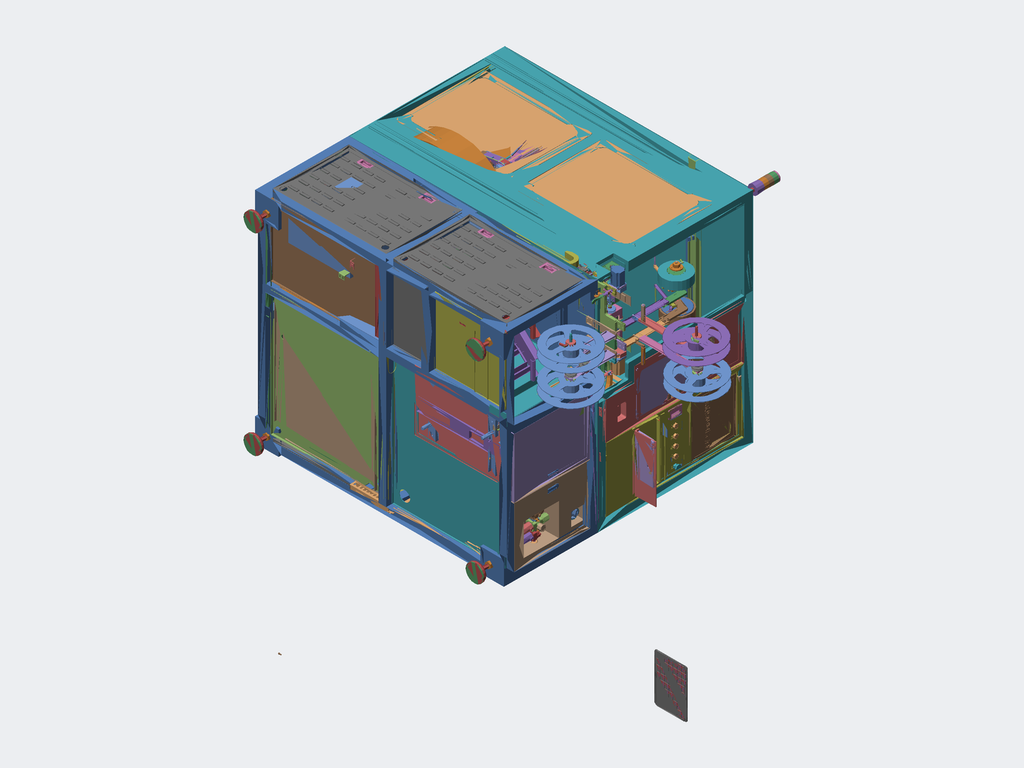Assembly | STEP file | 717 different items | 1668 placed
Parts list (item | name | quantity | parent item | size | volume), first 404 of 717 items:
1 | 11- Drag Chain 202811_2 | x3 | in 11-°ü×°11 | - | -
2 | 11- Filter C11 | x1 | - | - | -
3 | 11- M3-25 Hex Socket Countersunk Screw11_BOX-CBF3-25 | x1 | - | - | -
4 | 11- M3-5 Hex Socket Round Head Screw11_BCB3-5 | x5 | - | - | -
5 | 11- M4-10 Hex Socket Countersunk Screw11_BOX-CBF4-10 | x1 | - | - | -
6 | 11- M4-12 Hex Socket Countersunk Screw11_BOX-CBF4-12 | x2 | - | - | -
7 | 11- M4-20 Hex Socket Countersunk Screw11_BOX-CBF4-20 | x1 | - | - | -
8 | 11- M5 Nut CW11 | x2 | - | - | -
9 | 11- M5-12 Hex Socket Countersunk Screw11_BOX-CBF5-12 | x1 | - | - | -
10 | 11- M5-15 Hex Socket Countersunk Screw11_BOX-CBF5-15 | x1 | - | - | -
11 | 11- M5-30 Hex Socket Countersunk Screw11_BOX-CBF5-30 | x1 | - | - | -
12 | 11- M5-40 Hex Socket Countersunk Screw CW11_BOX-CBF5-40 | x2 | - | - | -
13 | 11- M5-40 Hex Socket Countersunk Screw11_BOX-CBF5-40 | x2 | - | - | -
14 | 11- M6-40 Hex Socket Countersunk Screw11_BOX-CBF6-40 | x1 | - | - | -
15 | 11- Mirror 99-JX-009-98-9865-998-1.·11 | x1 | - | - | -
16 | 11- Mirror 99-UWUAN94_B-98-9865-998-1.·11_UWUAN94-B | x1 | - | - | -
17 | 11- Mirror 99-XJX-006-98-9865-998-1.·11 | x1 | - | - | -
18 | 11- Mirror AJST4-5511 | x2 | - | - | -
19 | 11- Mirror ARM_MC01-S311 | x1 | in 11- Mirror MC01-S311 | - | -
20 | 11- Mirror AWY6_2511 | x1 | - | - | -
21 | 11- Mirror B676ZZ11_B676ZZ | x1 | - | - | -
22 | 11- Mirror B6800ZZ11_B6800ZZ | x4 | - | - | -
23 | 11- Mirror B686ZZ11_B686ZZ | x1 | - | - | -
24 | 11- Mirror B688ZZ11 | x2 | in 11- Mirror Roller111 | - | -
25 | 11- Mirror B698ZZ11_B698ZZ | x1 | - | - | -
26 | 11- Mirror BASE_MC01-S311 | x1 | in 11- Mirror MC01-S311 | - | -
27 | 11- Mirror BSPO4_15b11 | x2 | in 11- Mirror BSPO4_1511, 11- Mirror BSPO4_15111 | - | -
28 | 11- Mirror BZ-00811 | x1 | - | - | -
29 | 11- Mirror Body_A_CDQSB16_10D_A93_0_11 | x2 | in 11- Mirror CDQ16-10D11, 11- Mirror CDQ16-10D111 | - | -
30 | 11- Mirror CC-MCH-6.5-50-100-100w-6-5011 | x2 | - | - | -
31 | 11- Mirror CLDMC6_20_B_111 | x2 | in 11- Mirror CLDMC6_20_B11, 11- Mirror CLDMC6_20_B111 | - | -
32 | 11- Mirror CLDMC6_20_B_211 | x2 | in 11- Mirror CLDMC6_20_B11, 11- Mirror CLDMC6_20_B111 | - | -
33 | 11- Mirror CLMPLV_CLDM5-25-B11 | x2 | in 11- Mirror CLDM5-25-B11, 11- Mirror CLDM5-25-B111 | - | -
34 | 11- Mirror CLMP_MC01-S311 | x2 | in 11- Mirror MC01-S311 | - | -
35 | 11- Mirror FG-B00111 | x1 | - | - | -
36 | 11- Mirror FG-B00211 | x2 | - | - | -
37 | 11- Mirror FG-B00311 | x3 | - | - | -
38 | 11- Mirror FG-B00411 | x3 | - | - | -
39 | 11- Mirror FG-B00511 | x1 | - | - | -
40 | 11- Mirror FG-B00611 | x2 | - | - | -
41 | 11- Mirror FG-B00811 | x1 | - | - | -
42 | 11- Mirror FG-B00911 | x1 | - | - | -
43 | 11- Mirror FG-B01011 | x1 | - | - | -
44 | 11- Mirror FG-B01111 | x2 | - | - | -
45 | 11- Mirror FG-B01211 | x1 | - | - | -
46 | 11- Mirror FG-B01311 | x2 | - | - | -
47 | 11- Mirror FG-B01411 | x1 | - | - | -
48 | 11- Mirror FG-B01611 | x2 | - | - | -
49 | 11- Mirror FG-B01711 | x2 | - | - | -
50 | 11- Mirror FG-B01811 | x1 | - | - | -
51 | 11- Mirror FG-B01911 | x3 | - | - | -
52 | 11- Mirror FG-B02011 | x2 | - | - | -
53 | 11- Mirror FG-B02111 | x2 | - | - | -
54 | 11- Mirror FG-B02211 | x2 | - | - | -
55 | 11- Mirror FG-B02311 | x2 | - | - | -
56 | 11- Mirror FG-B02411 | x2 | - | - | -
57 | 11- Mirror FG-B02511 | x2 | - | - | -
58 | 11- Mirror FG-B02611 | x2 | - | - | -
59 | 11- Mirror FG-B02711 | x2 | - | - | -
60 | 11- Mirror FG-B02811 | x2 | - | - | -
61 | 11- Mirror FG-B03011 | x2 | - | - | -
62 | 11- Mirror FG-B03211 | x2 | - | - | -
63 | 11- Mirror FG-B03311 | x1 | - | - | -
64 | 11- Mirror FG-B03411 | x2 | - | - | -
65 | 11- Mirror FG-B03611 | x1 | - | - | -
66 | 11- Mirror FG-B03711 | x1 | - | - | -
67 | 11- Mirror FG-B03811 | x1 | - | - | -
68 | 11- Mirror FG-B03911 | x1 | - | - | -
69 | 11- Mirror FG-B04011 | x1 | - | - | -
70 | 11- Mirror FG-B04111 | x1 | - | - | -
71 | 11- Mirror FG-B04211 | x1 | - | - | -
72 | 11- Mirror FG-B04311 | x1 | - | - | -
73 | 11- Mirror FG-B04411 | x1 | - | - | -
74 | 11- Mirror FG-B04511 | x1 | - | - | -
75 | 11- Mirror FG-B04611 | x1 | - | - | -
76 | 11- Mirror FG-B04711 | x1 | - | - | -
77 | 11- Mirror FG-B04811 | x1 | - | - | -
78 | 11- Mirror FG-B04911 | x1 | - | - | -
79 | 11- Mirror FG-B05011 | x1 | - | - | -
80 | 11- Mirror FG-B05111 | x1 | - | - | -
81 | 11- Mirror FG-B05211 | x1 | - | - | -
82 | 11- Mirror FG-B05311 | x1 | - | - | -
83 | 11- Mirror FG-B05411 | x1 | - | - | -
84 | 11- Mirror FG-B05511 | x1 | - | - | -
85 | 11- Mirror FG-B05611 | x1 | - | - | -
86 | 11- Mirror FG-B05711 | x1 | - | - | -
87 | 11- Mirror FG-B05811 | x1 | - | - | -
88 | 11- Mirror FG-B05911 | x2 | - | - | -
89 | 11- Mirror FG-B06011 | x1 | - | - | -
90 | 11- Mirror FG-B06711 | x1 | - | - | -
91 | 11- Mirror FG-B06811 | x1 | in 11- Mirror Roller111 | - | -
92 | 11- Mirror FG-B06911 | x1 | in 11- Mirror Roller111 | - | -
93 | 11- Mirror FG-B07111 | x3 | - | - | -
94 | 11- Mirror FG-B07211 | x1 | - | - | -
95 | 11- Mirror FG-B07311 | x1 | - | - | -
96 | 11- Mirror FG-B07411 | x1 | - | - | -
97 | 11- Mirror FG-B07511 | x2 | - | - | -
98 | 11- Mirror FG-B07611 | x2 | - | - | -
99 | 11- Mirror FG-B07711 | x1 | - | - | -
100 | 11- Mirror FG-B07811 | x2 | - | - | -
101 | 11- Mirror FG-B07911 | x1 | - | - | -
102 | 11- Mirror FG-B08011 | x2 | - | - | -
103 | 11- Mirror FG-B08111 | x1 | - | - | -
104 | 11- Mirror FG-B08211 | x2 | - | - | -
105 | 11- Mirror FG-B08311 | x1 | - | - | -
106 | 11- Mirror FG-B08611 | x1 | - | - | -
107 | 11- Mirror FG-B08711 | x2 | - | - | -
108 | 11- Mirror FG-B08811 | x1 | - | - | -
109 | 11- Mirror FG-B08911 | x1 | - | - | -
110 | 11- Mirror FG-BZ02111 | x1 | - | - | -
111 | 11- Mirror FG-BZ02211 | x1 | - | - | -
112 | 11- Mirror FG-BZ02311 | x1 | - | - | -
113 | 11- Mirror FG-BZ02411 | x1 | - | - | -
114 | 11- Mirror FG-BZ02511 | x1 | - | - | -
115 | 11- Mirror FG-SB00411 | x1 | in 11- Media Pick-up Nozzle Assembly-A11 | - | -
116 | 11- Mirror FG-SB00511 | x1 | in 11- Media Pick-up Nozzle Assembly-A11 | - | -
117 | 11- Mirror FG-SB00611 | x1 | in 11- Media Pick-up Nozzle Assembly-A11 | - | -
118 | 11- Mirror FG-SB00711 | x3 | in 11- Media Pick-up Nozzle Assembly-A11 | - | -
119 | 11- Mirror FG-SB00811 | x1 | in 11- Media Pick-up Nozzle Assembly-A11 | - | -
120 | 11- Mirror FG-SB00911 | x1 | in 11- Media Pick-up Nozzle Assembly-A11 | - | -
121 | 11- Mirror FG-SZ01811 | x1 | - | - | -
122 | 11- Mirror FJTM4_0_7_413part111 | x2 | in 11- Mirror FJTM4_0_7_411, 11- Mirror FJTM4_0_7_4111 | - | -
123 | 11- Mirror FJTM4_0_7_413part211 | x2 | in 11- Mirror FJTM4_0_7_411, 11- Mirror FJTM4_0_7_4111 | - | -
124 | 11- Mirror FL6800ZZ11_FL6800ZZ | x2 | - | - | -
125 | 11- Mirror FL6902ZZ11 | x2 | - | - | -
126 | 11- Mirror GYJJ-013-q11 | x3 | - | - | -
127 | - | x4 | in 11- Mirror HTPA24S3M060_A_P811, 11- Mirror HTPA24S3M060_A_P8111 | - | -
128 | 11- Mirror HANDLE_MC01-S311 | x1 | in 11- Mirror MC01-S311 | - | -
129 | 11- Mirror HGR1511 | x2 | in 11- Mirror HGW15CC11, 11- Mirror HGW15CC111 | - | -
130 | 11- Mirror HGW1511 | x4 | in 11- Mirror HGW15CC11, 11- Mirror HGW15CC111 | - | -
131 | 11- Mirror HLB1011_HLB10 | x1 | - | - | -
132 | 11- Mirror HTPA24S3M060_A_P8_a11 | x2 | in 11- Mirror HTPA24S3M060_A_P811, 11- Mirror HTPA24S3M060_A_P8111 | - | -
133 | 11- Mirror KEYENCE-PQ0211 | x2 | - | - | -
134 | 11- Mirror LINK_MC01-S311 | x1 | in 11- Mirror MC01-S311 | - | -
135 | 11- Mirror LMU6-A11_C-LMU6 | x3 | in 11- Media Pick-up Nozzle Assembly-A11 | - | -
136 | 11- Mirror LMU_N811 | x3 | - | - | -
137 | 11- Mirror M3-25 Hex Socket Countersunk Screw11_BOX-CBF3-25 | x1 | - | - | -
138 | 11- Mirror M3-5 Hex Socket Round Head Screw11_BCB3-5 | x5 | - | - | -
139 | 11- Mirror M4x0_7A11 | x2 | in 11- Mirror BSPO4_1511, 11- Mirror BSPO4_15111 | - | -
140 | 11- Mirror M5-15 Hex Socket Countersunk Screw11_BOX-CBF5-15 | x1 | - | - | -
141 | 11- Mirror M5-40 Hex Socket Countersunk Screw11_BOX-CBF5-40 | x2 | - | - | -
142 | 11- Mirror M6-40 Hex Socket Countersunk Screw11_BOX-CBF6-40 | x1 | - | - | -
143 | 11- Mirror MANIFOLD_SOLID_BREP_3911 | x6 | in 11- Mirror SAND94F7H98T_ASM11, 11- Mirror SAND94F7H98T_ASM111 | - | -
144 | 11- Mirror MANIFOLD_SOLID_BREP_4011 | x2 | in 11- Mirror SAND94F7H98T_ASM11, 11- Mirror SAND94F7H98T_ASM111 | - | -
145 | 11- Mirror MBR58_3_P811 | x2 | - | - | -
146 | 11- Mirror MSB6_2011 | x1 | - | - | -
147 | 11- Mirror MSB8_1011_MSB8-10 | x1 | - | - | -
148 | 11- Mirror Mirror FG-B01911 | x1 | - | - | -
149 | 11- Mirror Mirror FG-B07111 | x1 | - | - | -
150 | 11- Mirror Mirror FG-B07511 | x1 | - | - | -
151 | 11- Mirror Mirror FG-B07611 | x1 | - | - | -
152 | 11- Mirror NAT-M6_MC01-S311 | x2 | in 11- Mirror MC01-S311 | - | -
153 | 11- Mirror NEZI-M6x40L_MC01-S311 | x1 | in 11- Mirror MC01-S311 | - | -
154 | 11- Mirror NEZIPART_CLDM5-25-B11 | x2 | in 11- Mirror CLDM5-25-B11, 11- Mirror CLDM5-25-B111 | - | -
155 | 11- Mirror Rod_A_CDQSB16_10D_A93_0_11 | x2 | in 11- Mirror CDQ16-10D11, 11- Mirror CDQ16-10D111 | - | -
156 | 11- Mirror SFJW6-31-M3-N311 | x3 | in 11- Media Pick-up Nozzle Assembly-A11 | - | -
157 | 11- Mirror SSEBT13_7011 | x2 | in 11- Mirror SSEBT13-7011 | - | -
158 | 11- Mirror STWN1511 | x1 | - | - | -
159 | 11- Mirror STWN811 | x2 | in 11- Mirror Roller111 | - | -
160 | 11- Mirror UF8-15-A11_UV8-15 | x1 | in 11- Media Pick-up Nozzle Assembly-A11 | - | -
161 | 11- Mirror WT8_1511 | x1 | - | - | -
162 | 11- Mirror b_SEB1011 | x2 | in 11- Mirror SEBL10_4011, 11- Mirror SEBL10_40111 | - | -
163 | 11- Mirror b_SSEBT1311 | x2 | in 11- Mirror SSEBT13-7011 | - | -
164 | 11- Mirror c-ssmt6-100011 | x2 | - | - | -
165 | 11- Mirror r_SEBL10_4011 | x2 | in 11- Mirror SEBL10_4011, 11- Mirror SEBL10_40111 | - | -
166 | 11- Mirror roller-HSG11 | x2 | - | - | -
167 | 11- Mirror yk60hb86-04a11 | x1 | - | - | -
168 | 11- Optics Valley MISUMI-KES3-1511 | x1 | - | - | -
169 | 11- Optics Valley SS11111 | x2 | - | - | -
170 | 11- Optics Valley SS11411 | x1 | - | - | -
171 | 11-100GF-RC11 | x1 | in 11-200YB03_ASM-111 | 159.399 x 104.797 x 116.9 mm | 1389549 mm3
172 | 11-100YB200G11 | x1 | in 11-200YB03_ASM-111 | 105.972 x 105.485 x 221 mm | 385712 mm3
173 | 11-123211 | x2 | - | 450 x 380 x 10 mm | 1708660 mm3
174 | - | x1 | - | 80 x 80 x 151 mm | 637905 mm3
175 | - | x1 | - | - | -
176 | 11-6060-21411 | x1 | - | 62 x 44 x 264 mm | 101240 mm3
177 | - | x1 | - | - | -
178 | - | x1 | - | - | -
179 | - | x1 | - | - | -
180 | - | x1 | - | - | -
181 | - | x1 | - | - | -
182 | - | x2 | in 11-COMPANY_A Upper Frame Cover.·11 | 50 x 10 x 14 mm | 4964 mm3
183 | - | x2 | in 11-COMPANY_A Upper Frame Cover.·11 | 50 x 14 x 14 mm | 5525 mm3
184 | - | x1 | - | - | -
185 | - | x1 | in 11-COMPANY_A Upper Frame Cover.·11 | - | -
186 | 11-ACA-0806-1_BodyCW11_HI | x2 | in 11-ACA-0806-1CW11_HI | 8 x 50 x 8 mm | 1845 mm3
187 | 11-ACA-0806-1_NTCW11_HI | x4 | in 11-ACA-0806-1CW11_HI | 11 x 4 x 12.325 mm | 245.478 mm3
188 | 11-ACA2020-311 | x4 | - | 26 x 127.5 x 29.132 mm | 35458 mm3
189 | 11-AJST4-5511 | x2 | - | 70 x 8.083 x 7 mm | 1036 mm3
190 | 11-ARM_MC01-S311 | x1 | in 11-MC01-S311 | 68.35 x 24.739 x 11.4 mm | 4057 mm3
191 | 11-ASL5-M511 | x1 | - | 28.6 x 30 x 12.5 mm | 2571 mm3
192 | 11-AWY6_2511 | x1 | - | 26.2 x 6 x 6 mm | 169.712 mm3
193 | 11-B6800ZZ11_B6800ZZ | x2 | - | 5 x 19 x 19 mm | 1010 mm3
194 | 11-B686ZZ11_B686ZZ | x2 | in 11-°ü×°11 | 5 x 13 x 13 mm | 508.574 mm3
195 | 11-B688ZZ11 | x2 | in 11-Roller11 | 5 x 16 x 16 mm | 730.663 mm3
196 | 11-B6902ZZ11_B6902ZZ | x2 | - | 7 x 28 x 28 mm | 2801 mm3
197 | 11-B698ZZ11_B698ZZ | x1 | - | 6 x 19 x 19 mm | 1232 mm3
198 | 11-BASE_MC01-S311 | x1 | in 11-MC01-S311 | 37 x 25.5 x 36 mm | 4977 mm3
199 | 11-BSPO4_15b11 | x2 | in 11-BSPO4_1511 | 15 x 4 x 4 mm | 171.383 mm3
200 | 11-Base1111 | x2 | - | 290.067 x 170 x 310 mm | 1578242 mm3
201 | 11-Body_A_CDQSB16_10D_A93_0_11 | x2 | in 11-CDQ16-10D11 | 29 x 29 x 32 mm | 21093 mm3
202 | 11-CB5_15_1-ab11 | x18 | in 11-KDST12-ab11_KDST12 | 20 x 8.5 x 8.5 mm | 539.598 mm3
203 | 11-CC-MCH-6.5-50-100-100w-6-5011 | x2 | - | 6.5 x 6.5 x 70 mm | 1785 mm3
204 | 11-CLDMC6_20_B_111 | x4 | in 11-CLDMC6_20_B11 | 10 x 45.8 x 10 mm | 2201 mm3
205 | 11-CLDMC6_20_B_211 | x4 | in 11-CLDMC6_20_B11 | 36.5 x 25 x 13 mm | 3149 mm3
206 | 11-CLMPLV_CLDM5-25-B11 | x2 | in 11-CLDM5-25-B11 | 51.5 x 31 x 13 mm | 5282 mm3
207 | 11-CLMP_MC01-S311 | x2 | in 11-MC01-S311 | 18.4 x 3.9 x 15.2 mm | 446.915 mm3
208 | 11-CX-442 (Panasonic)11 | x2 | - | - | -
209 | 11-Cover11111 | x2 | - | - | -
210 | 11-Cover21111 | x2 | - | 305.265 x 4 x 124.613 mm | 9765 mm3
211 | 11-Cover31111 | x2 | - | 105.323 x 67.359 x 38.98 mm | 17481 mm3
212 | 11-Cover41111 | x2 | - | 127.366 x 293 x 68 mm | 86944 mm3
213 | 11-DHJ-LR-144X1911 | x4 | - | 144 x 19 x 41 mm | 51924 mm3
214 | 11-EE-SX674A11 | x3 | - | 13.6 x 27.7 x 15.5 mm | 2495 mm3
215 | 11-EG15_RAIL_170CW11 | x1 | in 11-EGH15CA1R200ZOC11 | 15 x 12.5 x 200 mm | 31138 mm3
216 | 11-EGH15CA_BLOCK_2CW11 | x2 | in 11-EGH15CA1R200ZOC11 | 34 x 19.5 x 56.8 mm | 30383 mm3
217 | 11-F-ACA10LM11 | x2 | - | 15.4 x 16 x 14 mm | 1343 mm3
218 | 11-F12906-LQ-STBB5_35bA11 | x3 | - | 38.5 x 9.2 x 8 mm | 847.17 mm3
219 | 11-F12906-LQ-XZQG1A11 | x2 | in 11-F12906-LQ-AIRTAC-HRQ30-A-G(DS1-H)A11 | 195.5 x 57 x 191 mm | 392334 mm3
220 | 11-F12906-LQ-XZQG2A11 | x2 | in 11-F12906-LQ-AIRTAC-HRQ30-A-G(DS1-H)A11 | 42 x 4 x 5.1 mm | 360.74 mm3
221 | 11-F12906-LQ-XZQG3A11 | x2 | in 11-F12906-LQ-AIRTAC-HRQ30-A-G(DS1-H)A11 | 42 x 4 x 5.1 mm | 360.74 mm3
222 | 11-FCG-ZJ10011 | x1 | in 11-200YB03_ASM-111 | 19 x 64 x 64 mm | 16815 mm3
223 | 11-FG Emergency Stop Switch (Red) 22mm.11 | x1 | - | - | -
224 | 11-FG Guangyu2222AN-00311 | x1 | - | - | -
225 | 11-FG Push Button Switch (White) 22mm.11 | x4 | - | - | -
226 | 11-FG-00911 | x1 | in 11- Acrylic Door 2.·11 | 618 x 900 x 5 mm | 2751412 mm3
227 | 11-FG-01011 | x1 | - | 300 x 370 x 5 mm | 531993 mm3
228 | 11-FG-B00111 | x1 | - | 20 x 25 x 97.4 mm | 30314 mm3
229 | 11-FG-B00211 | x2 | - | 20 x 25 x 96.4 mm | 29627 mm3
230 | 11-FG-B00311 | x3 | - | 127 x 10 x 5 mm | 4266 mm3
231 | 11-FG-B00411 | x3 | - | 8 x 8 x 137 mm | 6844 mm3
232 | 11-FG-B00511 | x1 | - | 15 x 31 x 25 mm | 8369 mm3
233 | 11-FG-B00611 | x1 | - | 13.5 x 8.4 x 419 mm | 44557 mm3
234 | 11-FG-B00711 | x1 | - | 60 x 67.3 x 10 mm | 36302 mm3
235 | 11-FG-B00811 | x1 | - | 20 x 50 x 97.4 mm | 60152 mm3
236 | 11-FG-B00911 | x1 | - | 20 x 50 x 96.4 mm | 61320 mm3
237 | 11-FG-B01011 | x1 | - | 15 x 31 x 50 mm | 19389 mm3
238 | 11-FG-B01111 | x1 | - | 13.5 x 8.4 x 426 mm | 45040 mm3
239 | 11-FG-B01211 | x1 | - | 34 x 95 x 45 mm | 11150 mm3
240 | 11-FG-B01311 | x1 | - | 29 x 16.2 x 16.2 mm | 699.681 mm3
241 | 11-FG-B01411 | x1 | - | 8 x 21.5 x 55 mm | 827.809 mm3
242 | 11-FG-B01511 | x3 | - | 50 x 47.5 x 15 mm | 25829 mm3
243 | 11-FG-B01611 | x2 | - | 11 x 10 x 17 mm | 1460 mm3
244 | 11-FG-B01711 | x2 | - | 4 x 4 x 155 mm | 1945 mm3
245 | 11-FG-B01811 | x1 | - | 127 x 237 x 10 mm | 161294 mm3
246 | 11-FG-B01911 | x1 | - | 165 x 10 x 65 mm | 66276 mm3
247 | 11-FG-B02011 | x2 | - | 34 x 34 x 7 mm | 7241 mm3
248 | 11-FG-B02111 | x2 | - | 40.5 x 70 x 71 mm | 84307 mm3
249 | 11-FG-B02211 | x2 | - | 8 x 82 x 55 mm | 15645 mm3
250 | 11-FG-B02311 | x2 | - | 14 x 55 x 108 mm | 52508 mm3
251 | 11-FG-B02411 | x2 | - | 53 x 9 x 15 mm | 5874 mm3
252 | 11-FG-B02511 | x2 | - | 50 x 55 x 30 mm | 33514 mm3
253 | 11-FG-B02611 | x2 | - | 70 x 8 x 8 mm | 2907 mm3
254 | 11-FG-B02711 | x2 | - | 55 x 24 x 25 mm | 23943 mm3
255 | 11-FG-B02811 | x2 | - | 55 x 25 x 8 mm | 9529 mm3
256 | 11-FG-B02911 | x1 | - | 20 x 25 x 97.4 mm | 29767 mm3
257 | 11-FG-B03011 | x2 | - | 55 x 30 x 6 mm | 6845 mm3
258 | 11-FG-B03111 | x1 | - | 1.6 x 16 x 110 mm | 2770 mm3
259 | 11-FG-B03211 | x2 | - | 18.5 x 14.8 x 55 mm | 13198 mm3
260 | 11-FG-B03311 | x2 | - | 32 x 55 x 25 mm | 31224 mm3
261 | 11-FG-B03411 | x2 | - | 73 x 164 x 62 mm | 23088 mm3
262 | 11-FG-B03511 | x1 | - | 60 x 67.3 x 10 mm | 35980 mm3
263 | 11-FG-B03611 | x1 | - | 35 x 90 x 10 mm | 26239 mm3
264 | 11-FG-B03711 | x1 | - | 60 x 69.55 x 10 mm | 25100 mm3
265 | 11-FG-B03811 | x1 | - | 46 x 20 x 9 mm | 5580 mm3
266 | 11-FG-B03911 | x1 | - | 70 x 15 x 10.45 mm | 9294 mm3
267 | 11-FG-B04011 | x1 | - | 13 x 13 x 12.6 mm | 939.65 mm3
268 | 11-FG-B04111 | x1 | - | 30 x 30 x 15 mm | 6699 mm3
269 | 11-FG-B04211 | x1 | - | 13 x 13 x 19 mm | 1362 mm3
270 | 11-FG-B04311 | x1 | - | 13 x 13 x 2 mm | 108.385 mm3
271 | 11-FG-B04411 | x1 | - | 16 x 193.5 x 14 mm | 10709 mm3
272 | 11-FG-B045-(Standard Gear)11 | x2 | - | - | -
273 | 11-FG-B04611 | x2 | - | 35 x 35 x 16 mm | 6298 mm3
274 | 11-FG-B04711 | x1 | - | 100 x 40 x 12 mm | 42920 mm3
275 | 11-FG-B04811 | x1 | - | 40 x 300 x 10 mm | 115513 mm3
276 | 11-FG-B04911 | x1 | - | 107.65 x 192.793 x 12 mm | 106173 mm3
277 | 11-FG-B05011 | x1 | - | 9.8 x 44.825 x 230.182 mm | 35809 mm3
278 | 11-FG-B05111 | x1 | - | 6 x 6 x 135 mm | 3802 mm3
279 | 11-FG-B05211 | x1 | - | 50 x 45 x 12 mm | 12836 mm3
280 | 11-FG-B05311 | x1 | - | 160 x 160 x 5 mm | 93587 mm3
281 | 11-FG-B05411 | x1 | - | 76 x 76 x 19 mm | 36918 mm3
282 | 11-FG-B05511 | x1 | - | 90 x 90 x 10 mm | 52768 mm3
283 | 11-FG-B05611 | x1 | - | 66 x 66 x 25 mm | 31855 mm3
284 | 11-FG-B05711 | x1 | - | 20 x 20 x 147 mm | 20612 mm3
285 | 11-FG-B05811 | x1 | - | 40 x 400 x 12 mm | 182663 mm3
286 | 11-FG-B05911 | x3 | - | 50 x 47.5 x 9 mm | 15360 mm3
287 | 11-FG-B06011 | x3 | - | 20 x 20 x 169.5 mm | 19381 mm3
288 | 11-FG-B06111 | x2 | - | 40 x 200 x 10 mm | 76186 mm3
289 | 11-FG-B06211 | x2 | - | 60 x 300 x 12 mm | 199770 mm3
290 | 11-FG-B06611 | x2 | - | 40 x 20 x 10 mm | 5422 mm3
291 | 11-FG-B06711 | x1 | - | 80 x 12 x 10 mm | 7960 mm3
292 | 11-FG-B06811 | x1 | in 11-Roller11 | 20 x 20 x 100 mm | 19227 mm3
293 | 11-FG-B06911 | x1 | in 11-Roller11 | 8 x 8 x 111 mm | 5459 mm3
294 | 11-FG-B07111 | x1 | - | 29 x 11 x 19.5 mm | 3288 mm3
295 | 11-FG-B07211 | x1 | - | 240 x 1100 x 15 mm | 2663856 mm3
296 | 11-FG-B07311 | x2 | - | 15 x 80 x 73 mm | 13404 mm3
297 | 11-FG-B07411 | x1 | - | 265 x 317.5 x 137 mm | 178477 mm3
298 | 11-FG-B07511 | x1 | - | 14.5 x 6 x 419 mm | 26571 mm3
299 | 11-FG-B07611 | x1 | - | 14.5 x 6 x 369.8 mm | 23525 mm3
300 | 11-FG-B07711 | x1 | - | 8.2 x 40 x 20 mm | 919.559 mm3
301 | 11-FG-B07811 | x2 | - | 50.5 x 9.5 x 25 mm | 9037 mm3
302 | 11-FG-B07911 | x1 | - | 15 x 55 x 25 mm | 16309 mm3
303 | 11-FG-B08011 | x2 | - | 20 x 32.5 x 4 mm | 1470 mm3
304 | 11-FG-B08111 | x1 | - | 8.2 x 40 x 20 mm | 912.829 mm3
305 | 11-FG-B08211 | x2 | - | 10 x 35 x 3 mm | 935.086 mm3
306 | 11-FG-B08311 | x1 | - | 4 x 4 x 130 mm | 1631 mm3
307 | 11-FG-B08411 | x2 | - | 8 x 7 x 41 mm | 1772 mm3
308 | 11-FG-B08511 | x2 | - | 40 x 10 x 10 mm | 3274 mm3
309 | 11-FG-B08611 | x1 | - | 126 x 381.8 x 413.682 mm | 331589 mm3
310 | 11-FG-B08711 | x1 | in 11-°ü×°11 | 70 x 20 x 20 mm | 26205 mm3
311 | 11-FG-B08911 | x2 | in 11-°ü×°11 | 44 x 31 x 400 mm | 61704 mm3
312 | 11-FG-B09011 | x2 | in 11-°ü×°11 | 70 x 60 x 60 mm | 21228 mm3
313 | 11-FG-DB00111 | x1 | - | 1650 x 1450 x 20 mm | 31427316 mm3
314 | 11-FG-E00111 | x1 | - | 300 x 186 x 20 mm | 846486 mm3
315 | 11-FG-E00211 | x2 | - | 60 x 234 x 15 mm | 152627 mm3
316 | 11-FG-E00311 | x1 | - | 25 x 38 x 30 mm | 10262 mm3
317 | 11-FG-E00411 | x1 | - | 25 x 38 x 30 mm | 10226 mm3
318 | 11-FG-E00511 | x1 | - | 32 x 108 x 10 mm | 20715 mm3
319 | 11-FG-E00611 | x1 | - | 80 x 30 x 12 mm | 11899 mm3
320 | 11-FG-E00711 | x1 | - | 10 x 11.547 x 52 mm | 1820 mm3
321 | 11-FG-E00811 | x1 | - | 67 x 44 x 9 mm | 18765 mm3
322 | 11-FG-E00911 | x1 | - | 32 x 40 x 10 mm | 10413 mm3
323 | 11-FG-E01011 | x1 | - | 145 x 60 x 15 mm | 112264 mm3
324 | 11-FG-E01111 | x1 | - | 100 x 15 x 200 mm | 285807 mm3
325 | 11-FG-E01211 | x1 | - | 85 x 20 x 29 mm | 44302 mm3
326 | 11-FG-E01311 | x2 | - | 45 x 40 x 16 mm | 15803 mm3
327 | 11-FG-E01411 | x1 | - | 28 x 12 x 43 mm | 8595 mm3
328 | 11-FG-E01511 | x1 | - | 180 x 70 x 17 mm | 176306 mm3
329 | 11-FG-E01611 | x2 | - | 18 x 35 x 13 mm | 6444 mm3
330 | 11-FG-E01711 | x4 | - | 31.54 x 53.795 x 3 mm | 2242 mm3
331 | 11-FG-E01811 | x1 | - | 42 x 45 x 8 mm | 10535 mm3
332 | 11-FG-E01911 | x2 | - | 30 x 79.5 x 10 mm | 21106 mm3
333 | 11-FG-E02011 | x4 | - | 70 x 96 x 12 mm | 42748 mm3
334 | 11-FG-E02111 | x4 | - | 15 x 40 x 53 mm | 17580 mm3
335 | 11-FG-E02211 | x2 | - | 110 x 120 x 14.5 mm | 149751 mm3
336 | 11-FG-E02311 | x2 | - | 150 x 120 x 12 mm | 207598 mm3
337 | 11-FG-E02411 | x1 | - | 180 x 70 x 17 mm | 168926 mm3
338 | 11-FG-E02511 | x8 | - | 15 x 40 x 15 mm | 6347 mm3
339 | 11-FG-E02611 | x2 | - | 21 x 46 x 5 mm | 3756 mm3
340 | 11-FG-E02711 | x1 | - | 38.1 x 20.5 x 8.5 mm | 5078 mm3
341 | 11-FG-E02811 | x1 | - | 10 x 25 x 3.5 mm | 772.571 mm3
342 | 11-FG-E02911 | x1 | - | 304 x 110 x 150 mm | 146272 mm3
343 | 11-FG-E03011 | x1 | - | 113 x 304 x 128 mm | 112726 mm3
344 | 11-FG-E03111 | x1 | - | 140 x 100 x 2 mm | 20888 mm3
345 | 11-FG-E03211 | x1 | - | 88 x 17 x 26 mm | 5114 mm3
346 | 11-FG-E03311 | x2 | - | 41 x 169.5 x 10 mm | 55320 mm3
347 | 11-FG-E03411 | x1 | - | 48 x 47 x 8 mm | 12187 mm3
348 | 11-FG-E03511 | x1 | - | 33 x 20.5 x 8.5 mm | 4296 mm3
349 | 11-FG-E03611 | x1 | - | 55 x 54 x 27 mm | 21102 mm3
350 | 11-FG-E03711 | x1 | - | 20 x 20 x 119 mm | 14191 mm3
351 | 11-FG-E03811 | x1 | - | 86 x 120 x 10 mm | 47794 mm3
352 | 11-FG-E03911 | x4 | - | 12 x 12 x 53 mm | 5607 mm3
353 | 11-FG-E04111 | x1 | - | 24 x 28 x 5 mm | 1836 mm3
354 | 11-FG-E04211 | x1 | - | 32 x 51.5 x 15 mm | 7039 mm3
355 | 11-FG-E04311 | x1 | - | 40 x 10 x 10 mm | 3121 mm3
356 | 11-FG-E04411 | x1 | - | 28 x 12 x 35 mm | 10850 mm3
357 | 11-FG-E04511 | x1 | - | 8 x 40 x 20 mm | 5456 mm3
358 | 11-FG-E04611 | x4 | - | 15 x 14 x 3 mm | 458.934 mm3
359 | 11-FG-GD00111 | x4 | - | 64 x 71.5 x 15 mm | 48677 mm3
360 | 11-FG-JJ-01211 | x1 | - | 586 x 623 x 57 mm | 744145 mm3
361 | 11-FG-JX00111 | x1 | - | 408 x 519 x 20 mm | 549034 mm3
362 | 11-FG-JX00211 | x1 | - | 1500 x 667.5 x 1700 mm | 66450953 mm3
363 | 11-FG-JX00411 | x1 | - | 408 x 519 x 106 mm | 749356 mm3
364 | 11-FG-JX00511 | x1 | - | 100 x 20 x 138 mm | 43680 mm3
365 | 11-FG-JX00611 | x1 | in 11-COMPANY_A Upper Frame Cover.·11 | 1500 x 1700 x 1065 mm | 13737481 mm3
366 | 11-FG-JX01211 | x1 | in 11- Acrylic Door 2.·11 | 688 x 948 x 20 mm | 601333 mm3
367 | 11-FG-JX01311 | x1 | - | 240 x 460 x 10 mm | 240740 mm3
368 | 11-FG-JX01411 | x1 | - | 485 x 460 x 10 mm | 675418 mm3
369 | 11-FG-JX01511 | x1 | - | 775 x 890 x 10 mm | 929885 mm3
370 | 11-FG-JX01611 | x1 | - | 775 x 521 x 24.03 mm | 906085 mm3
371 | 11-FG-JX01711 | x1 | - | 358 x 948 x 37 mm | 620154 mm3
372 | 11-FG-JX01911 | x1 | - | 415 x 630 x 2 mm | 516605 mm3
373 | 11-FG-JX02011 | x1 | - | 302 x 556 x 460 mm | 760169 mm3
374 | 11-FG-S00111 | x5 | - | 12 x 12 x 260 mm | 29196 mm3
375 | 11-FG-S00211 | x5 | - | 12 x 12 x 180 mm | 20348 mm3
376 | 11-FG-S00311 | x4 | - | 148 x 23 x 32 mm | 9076 mm3
377 | 11-FG-S00411 | x4 | - | 12 x 12 x 190 mm | 19715 mm3
378 | 11-FG-S00511 | x4 | - | 40 x 52 x 10 mm | 16876 mm3
379 | 11-FG-S00611 | x6 | - | 48 x 35 x 46 mm | 33562 mm3
380 | 11-FG-S00711 | x3 | - | 69 x 35 x 38.6 mm | 65613 mm3
381 | 11-FG-S00811 | x3 | - | 98 x 100 x 76 mm | 565928 mm3
382 | 11-FG-S00911 | x1 | - | 420 x 15 x 110 mm | 675941 mm3
383 | 11-FG-S01011 | x1 | - | 140 x 70 x 15 mm | 110078 mm3
384 | 11-FG-S01111 | x1 | - | 80 x 17 x 110 mm | 120634 mm3
385 | 11-FG-S01211 | x1 | - | 120 x 15 x 57 mm | 50768 mm3
386 | 11-FG-S01311 | x2 | - | 60 x 15 x 120 mm | 30172 mm3
387 | 11-FG-S01411 | x1 | - | 69 x 35 x 75.5 mm | 96843 mm3
388 | 11-FG-S01511 | x1 | - | 160 x 15 x 90 mm | 120227 mm3
389 | 11-FG-S01611 | x3 | - | 180 x 20 x 30 mm | 87134 mm3
390 | 11-FG-S01711 | x2 | - | 20 x 580 x 20 mm | 181847 mm3
391 | 11-FG-S02211 | x1 | - | 10 x 35 x 30 mm | 7793 mm3
392 | 11-FG-S02311 | x1 | - | 8 x 30 x 52 mm | 11750 mm3
393 | 11-FG-S02411 | x1 | - | 69 x 35 x 10 mm | 22541 mm3
394 | 11-FG-S02511 | x2 | - | 20 x 35 x 27.5 mm | 10097 mm3
395 | 11-FG-S02711 | x1 | - | 203 x 154 x 53 mm | 54999 mm3
396 | 11-FG-S02811 | x1 | - | 69 x 35 x 40.5 mm | 65665 mm3
397 | 11-FG-SB00111 | x2 | - | 200 x 170 x 148.5 mm | 3812542 mm3
398 | 11-FG-SB00211 | x1 | in 11- Media Pick-up Nozzle Assembly-A11 | 30 x 30 x 35 mm | 14894 mm3
399 | 11-FG-SB00311 | x1 | in 11- Media Pick-up Nozzle Assembly-A11 | 36 x 30 x 28 mm | 21147 mm3
400 | 11-FG-SB00411 | x1 | in 11- Media Pick-up Nozzle Assembly-A11 | 48.5 x 35 x 8 mm | 7407 mm3
401 | 11-FG-SB00511 | x1 | in 11- Media Pick-up Nozzle Assembly-A11 | 30 x 12 x 1.1 mm | 265.181 mm3
402 | 11-FG-SB00611 | x1 | in 11- Media Pick-up Nozzle Assembly-A11 | 35 x 12 x 1.1 mm | 324.378 mm3
403 | 11-FG-SB00711 | x5 | in 11- Media Pick-up Nozzle Assembly-A11 | 12 x 12 x 1.5 mm | 153.267 mm3
404 | 11-FG-SB00811 | x1 | in 11- Media Pick-up Nozzle Assembly-A11 | 35 x 50 x 7 mm | 10258 mm3